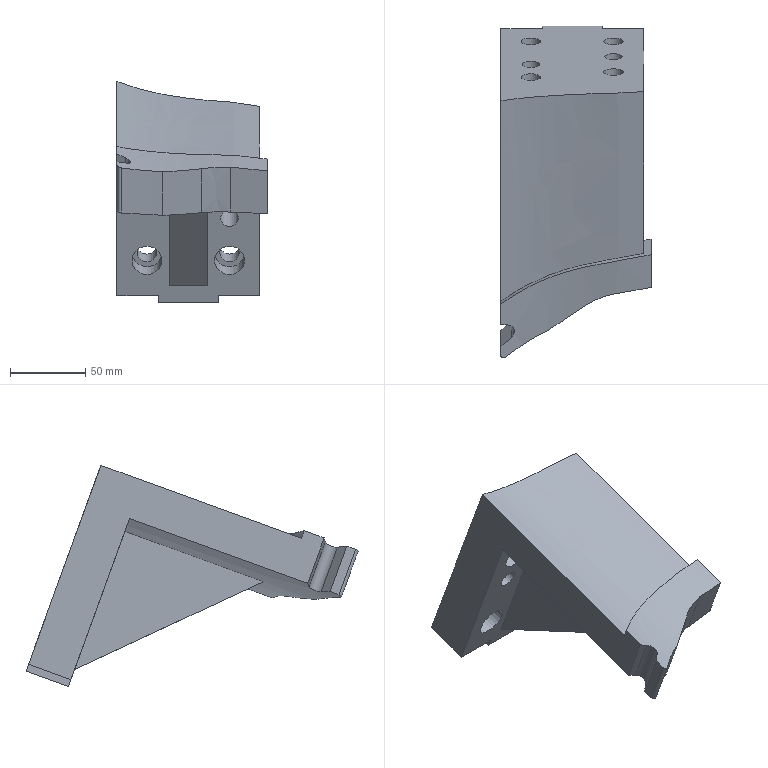Part | NX | features solid 2 | 1 solid | 40 faces | box 100 x 221.136 x 147.422 mm | volume 786388 mm3 | plane 18 | spline 11 | cylinder 11 | commonest cylinder face diameters 13 x4 20 x4 12 x2 10 x1